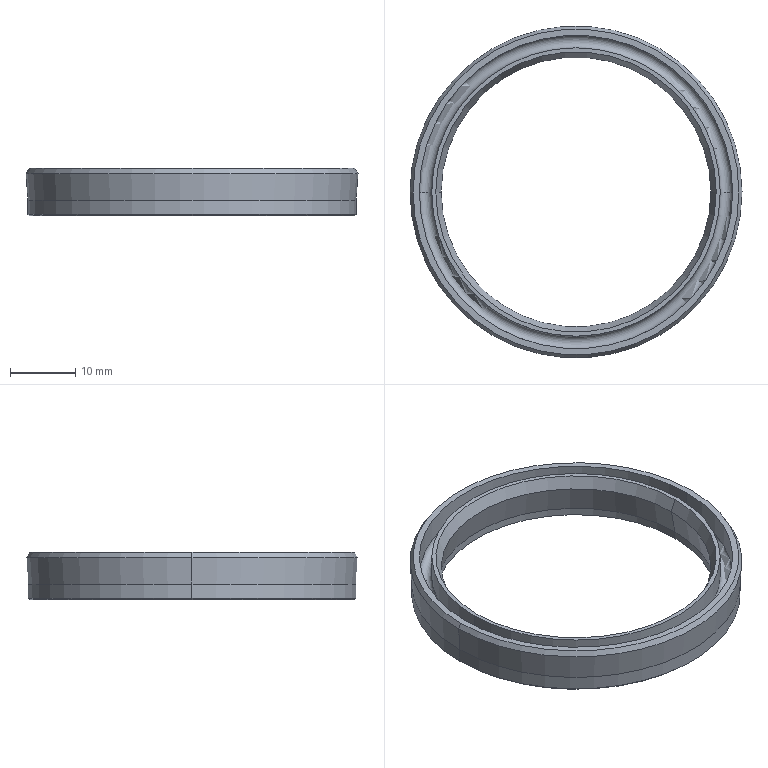Part | NX | features REVOLVE2 2 | 1 solid | 23 faces | box 50.8 x 50.8 x 7.235 mm | volume 3150 mm3 | cone 10 | cylinder 8 | plane 3 | torus 2 | commonest cylinder face diameters 42.799 x2 44.133 x2 47.943 x2 50.228 x2
STEP:
#1=CARTESIAN_POINT('',(25.114,0.,-1.59));
#2=VERTEX_POINT('',#1);
#3=CARTESIAN_POINT('',(-25.114,0.,-1.59));
#4=VERTEX_POINT('',#3);
#5=CARTESIAN_POINT('',(0.,0.,-1.59));
#6=DIRECTION('',(0.,0.,1.));
#7=DIRECTION('',(1.,0.,0.));
#8=AXIS2_PLACEMENT_3D('',#5,#6,#7);
#9=CIRCLE('',#8,25.114);
#10=EDGE_CURVE('',#2,#4,#9,.T.);
#11=ORIENTED_EDGE('',*,*,#10,.T.);
#12=CARTESIAN_POINT('',(-25.4,0.,2.465));
#13=VERTEX_POINT('',#12);
#14=CARTESIAN_POINT('',(-25.114,0.,-1.59));
#15=DIRECTION('',(-0.0703,0.,0.9975));
#16=VECTOR('',#15,1000.);
#17=LINE('',#14,#16);
#18=EDGE_CURVE('',#13,#4,#17,.F.);
#19=ORIENTED_EDGE('',*,*,#18,.F.);
#20=CARTESIAN_POINT('',(25.4,0.,2.465));
#21=VERTEX_POINT('',#20);
#22=CARTESIAN_POINT('',(0.,0.,2.465));
#23=DIRECTION('',(0.,0.,1.));
#24=DIRECTION('',(1.,0.,0.));
#25=AXIS2_PLACEMENT_3D('',#22,#23,#24);
#26=CIRCLE('',#25,25.4);
#27=EDGE_CURVE('',#21,#13,#26,.T.);
#28=ORIENTED_EDGE('',*,*,#27,.F.);
#29=CARTESIAN_POINT('',(25.114,0.,-1.59));
#30=DIRECTION('',(0.0703,0.,0.9975));
#31=VECTOR('',#30,1000.);
#32=LINE('',#29,#31);
#33=EDGE_CURVE('',#2,#21,#32,.T.);
#34=ORIENTED_EDGE('',*,*,#33,.F.);
#35=EDGE_LOOP('',(#11,#19,#28,#34));
#36=FACE_BOUND('',#35,.T.);
#37=CARTESIAN_POINT('',(0.,0.,-1.59));
#38=DIRECTION('',(0.,0.,1.));
#39=DIRECTION('',(-1.,0.,0.));
#40=AXIS2_PLACEMENT_3D('',#37,#38,#39);
#41=CONICAL_SURFACE('',#40,25.114,0.07036);
#42=ADVANCED_FACE('',(#36),#41,.T.);
#43=CARTESIAN_POINT('',(25.114,0.,-3.737));
#44=VERTEX_POINT('',#43);
#45=CARTESIAN_POINT('',(-25.114,0.,-3.737));
#46=VERTEX_POINT('',#45);
#47=CARTESIAN_POINT('',(0.,0.,-3.737));
#48=DIRECTION('',(0.,0.,1.));
#49=DIRECTION('',(1.,0.,0.));
#50=AXIS2_PLACEMENT_3D('',#47,#48,#49);
#51=CIRCLE('',#50,25.114);
#52=EDGE_CURVE('',#44,#46,#51,.T.);
#53=ORIENTED_EDGE('',*,*,#52,.T.);
#54=CARTESIAN_POINT('',(-25.114,0.,3.975));
#55=DIRECTION('',(0.,0.,1.));
#56=VECTOR('',#55,1000.);
#57=LINE('',#54,#56);
#58=EDGE_CURVE('',#46,#4,#57,.T.);
#59=ORIENTED_EDGE('',*,*,#58,.T.);
#60=ORIENTED_EDGE('',*,*,#10,.F.);
#61=CARTESIAN_POINT('',(25.114,0.,3.975));
#62=DIRECTION('',(0.,0.,1.));
#63=VECTOR('',#62,1000.);
#64=LINE('',#61,#63);
#65=EDGE_CURVE('',#2,#44,#64,.F.);
#66=ORIENTED_EDGE('',*,*,#65,.T.);
#67=EDGE_LOOP('',(#53,#59,#60,#66));
#68=FACE_BOUND('',#67,.T.);
#69=CARTESIAN_POINT('',(0.,0.,3.975));
#70=DIRECTION('',(0.,0.,1.));
#71=DIRECTION('',(-1.,0.,0.));
#72=AXIS2_PLACEMENT_3D('',#69,#70,#71);
#73=CYLINDRICAL_SURFACE('',#72,25.114);
#74=ADVANCED_FACE('',(#68),#73,.T.);
#75=CARTESIAN_POINT('',(24.876,0.,-3.975));
#76=VERTEX_POINT('',#75);
#77=CARTESIAN_POINT('',(-24.876,0.,-3.975));
#78=VERTEX_POINT('',#77);
#79=CARTESIAN_POINT('',(0.,0.,-3.975));
#80=DIRECTION('',(0.,0.,1.));
#81=DIRECTION('',(1.,0.,0.));
#82=AXIS2_PLACEMENT_3D('',#79,#80,#81);
#83=CIRCLE('',#82,24.876);
#84=EDGE_CURVE('',#76,#78,#83,.T.);
#85=ORIENTED_EDGE('',*,*,#84,.T.);
#86=CARTESIAN_POINT('',(-24.876,0.,-3.975));
#87=DIRECTION('',(-0.7071,0.,0.7071));
#88=VECTOR('',#87,1000.);
#89=LINE('',#86,#88);
#90=EDGE_CURVE('',#78,#46,#89,.T.);
#91=ORIENTED_EDGE('',*,*,#90,.T.);
#92=ORIENTED_EDGE('',*,*,#52,.F.);
#93=CARTESIAN_POINT('',(24.876,0.,-3.975));
#94=DIRECTION('',(0.7071,0.,0.7071));
#95=VECTOR('',#94,1000.);
#96=LINE('',#93,#95);
#97=EDGE_CURVE('',#44,#76,#96,.F.);
#98=ORIENTED_EDGE('',*,*,#97,.T.);
#99=EDGE_LOOP('',(#85,#91,#92,#98));
#100=FACE_BOUND('',#99,.T.);
#101=CARTESIAN_POINT('',(0.,0.,-3.975));
#102=DIRECTION('',(0.,0.,1.));
#103=DIRECTION('',(-1.,0.,0.));
#104=AXIS2_PLACEMENT_3D('',#101,#102,#103);
#105=CONICAL_SURFACE('',#104,24.876,0.7854);
#106=ADVANCED_FACE('',(#100),#105,.T.);
#107=CARTESIAN_POINT('',(-21.399,0.,-3.975));
#108=VERTEX_POINT('',#107);
#109=CARTESIAN_POINT('',(21.399,0.,-3.975));
#110=VERTEX_POINT('',#109);
#111=CARTESIAN_POINT('',(0.,0.,-3.975));
#112=DIRECTION('',(0.,0.,1.));
#113=DIRECTION('',(1.,0.,0.));
#114=AXIS2_PLACEMENT_3D('',#111,#112,#113);
#115=CIRCLE('',#114,21.399);
#116=EDGE_CURVE('',#108,#110,#115,.T.);
#117=ORIENTED_EDGE('',*,*,#116,.F.);
#118=CARTESIAN_POINT('',(-21.399,0.,-2.783));
#119=VERTEX_POINT('',#118);
#120=CARTESIAN_POINT('',(-21.399,0.,3.975));
#121=DIRECTION('',(0.,0.,1.));
#122=VECTOR('',#121,1000.);
#123=LINE('',#120,#122);
#124=EDGE_CURVE('',#108,#119,#123,.T.);
#125=ORIENTED_EDGE('',*,*,#124,.T.);
#126=CARTESIAN_POINT('',(21.399,0.,-2.783));
#127=VERTEX_POINT('',#126);
#128=CARTESIAN_POINT('',(0.,0.,-2.783));
#129=DIRECTION('',(0.,0.,1.));
#130=DIRECTION('',(1.,0.,0.));
#131=AXIS2_PLACEMENT_3D('',#128,#129,#130);
#132=CIRCLE('',#131,21.399);
#133=EDGE_CURVE('',#119,#127,#132,.T.);
#134=ORIENTED_EDGE('',*,*,#133,.T.);
#135=CARTESIAN_POINT('',(21.399,0.,3.975));
#136=DIRECTION('',(0.,0.,1.));
#137=VECTOR('',#136,1000.);
#138=LINE('',#135,#137);
#139=EDGE_CURVE('',#127,#110,#138,.F.);
#140=ORIENTED_EDGE('',*,*,#139,.T.);
#141=EDGE_LOOP('',(#117,#125,#134,#140));
#142=FACE_BOUND('',#141,.T.);
#143=CARTESIAN_POINT('',(0.,0.,3.975));
#144=DIRECTION('',(0.,0.,1.));
#145=DIRECTION('',(-1.,0.,0.));
#146=AXIS2_PLACEMENT_3D('',#143,#144,#145);
#147=CYLINDRICAL_SURFACE('',#146,21.399);
#148=ADVANCED_FACE('',(#142),#147,.F.);
#149=CARTESIAN_POINT('',(-20.637,0.,1.391));
#150=VERTEX_POINT('',#149);
#151=CARTESIAN_POINT('',(20.637,0.,1.391));
#152=VERTEX_POINT('',#151);
#153=CARTESIAN_POINT('',(0.,0.,1.391));
#154=DIRECTION('',(0.,0.,1.));
#155=DIRECTION('',(1.,0.,0.));
#156=AXIS2_PLACEMENT_3D('',#153,#154,#155);
#157=CIRCLE('',#156,20.637);
#158=EDGE_CURVE('',#150,#152,#157,.T.);
#159=ORIENTED_EDGE('',*,*,#158,.T.);
#160=CARTESIAN_POINT('',(20.637,0.,1.391));
#161=DIRECTION('',(0.1796,0.,-0.9837));
#162=VECTOR('',#161,1000.);
#163=LINE('',#160,#162);
#164=EDGE_CURVE('',#152,#127,#163,.T.);
#165=ORIENTED_EDGE('',*,*,#164,.T.);
#166=ORIENTED_EDGE('',*,*,#133,.F.);
#167=CARTESIAN_POINT('',(-20.637,0.,1.391));
#168=DIRECTION('',(-0.1796,0.,-0.9837));
#169=VECTOR('',#168,1000.);
#170=LINE('',#167,#169);
#171=EDGE_CURVE('',#119,#150,#170,.F.);
#172=ORIENTED_EDGE('',*,*,#171,.T.);
#173=EDGE_LOOP('',(#159,#165,#166,#172));
#174=FACE_BOUND('',#173,.T.);
#175=CARTESIAN_POINT('',(0.,0.,1.391));
#176=DIRECTION('',(0.,0.,-1.));
#177=DIRECTION('',(1.,0.,0.));
#178=AXIS2_PLACEMENT_3D('',#175,#176,#177);
#179=CONICAL_SURFACE('',#178,20.637,0.1806);
#180=ADVANCED_FACE('',(#174),#179,.F.);
#181=ORIENTED_EDGE('',*,*,#158,.F.);
#182=CARTESIAN_POINT('',(-21.447,0.,3.26));
#183=VERTEX_POINT('',#182);
#184=CARTESIAN_POINT('',(-21.447,0.,3.26));
#185=DIRECTION('',(-0.3976,0.,0.9176));
#186=VECTOR('',#185,1000.);
#187=LINE('',#184,#186);
#188=EDGE_CURVE('',#183,#150,#187,.F.);
#189=ORIENTED_EDGE('',*,*,#188,.F.);
#190=CARTESIAN_POINT('',(21.447,0.,3.26));
#191=VERTEX_POINT('',#190);
#192=CARTESIAN_POINT('',(0.,0.,3.26));
#193=DIRECTION('',(0.,0.,1.));
#194=DIRECTION('',(1.,0.,0.));
#195=AXIS2_PLACEMENT_3D('',#192,#193,#194);
#196=CIRCLE('',#195,21.447);
#197=EDGE_CURVE('',#183,#191,#196,.T.);
#198=ORIENTED_EDGE('',*,*,#197,.T.);
#199=CARTESIAN_POINT('',(21.447,0.,3.26));
#200=DIRECTION('',(0.3976,0.,0.9176));
#201=VECTOR('',#200,1000.);
#202=LINE('',#199,#201);
#203=EDGE_CURVE('',#152,#191,#202,.T.);
#204=ORIENTED_EDGE('',*,*,#203,.F.);
#205=EDGE_LOOP('',(#181,#189,#198,#204));
#206=FACE_BOUND('',#205,.T.);
#207=CARTESIAN_POINT('',(0.,0.,3.26));
#208=DIRECTION('',(0.,0.,1.));
#209=DIRECTION('',(-1.,0.,0.));
#210=AXIS2_PLACEMENT_3D('',#207,#208,#209);
#211=CONICAL_SURFACE('',#210,21.447,0.4089);
#212=ADVANCED_FACE('',(#206),#211,.F.);
#213=CARTESIAN_POINT('',(22.066,0.,-0.24));
#214=VERTEX_POINT('',#213);
#215=CARTESIAN_POINT('',(-22.066,0.,-0.24));
#216=VERTEX_POINT('',#215);
#217=CARTESIAN_POINT('',(0.,0.,-0.24));
#218=DIRECTION('',(0.,0.,1.));
#219=DIRECTION('',(1.,0.,0.));
#220=AXIS2_PLACEMENT_3D('',#217,#218,#219);
#221=CIRCLE('',#220,22.066);
#222=EDGE_CURVE('',#214,#216,#221,.T.);
#223=ORIENTED_EDGE('',*,*,#222,.T.);
#224=CARTESIAN_POINT('',(-22.066,0.,3.26));
#225=VERTEX_POINT('',#224);
#226=CARTESIAN_POINT('',(-22.066,0.,3.975));
#227=DIRECTION('',(0.,0.,1.));
#228=VECTOR('',#227,1000.);
#229=LINE('',#226,#228);
#230=EDGE_CURVE('',#216,#225,#229,.T.);
#231=ORIENTED_EDGE('',*,*,#230,.T.);
#232=CARTESIAN_POINT('',(22.066,0.,3.26));
#233=VERTEX_POINT('',#232);
#234=CARTESIAN_POINT('',(0.,0.,3.26));
#235=DIRECTION('',(0.,0.,1.));
#236=DIRECTION('',(1.,0.,0.));
#237=AXIS2_PLACEMENT_3D('',#234,#235,#236);
#238=CIRCLE('',#237,22.066);
#239=EDGE_CURVE('',#233,#225,#238,.T.);
#240=ORIENTED_EDGE('',*,*,#239,.F.);
#241=CARTESIAN_POINT('',(22.066,0.,3.975));
#242=DIRECTION('',(0.,0.,1.));
#243=VECTOR('',#242,1000.);
#244=LINE('',#241,#243);
#245=EDGE_CURVE('',#233,#214,#244,.F.);
#246=ORIENTED_EDGE('',*,*,#245,.T.);
#247=EDGE_LOOP('',(#223,#231,#240,#246));
#248=FACE_BOUND('',#247,.T.);
#249=CARTESIAN_POINT('',(0.,0.,3.975));
#250=DIRECTION('',(0.,0.,1.));
#251=DIRECTION('',(-1.,0.,0.));
#252=AXIS2_PLACEMENT_3D('',#249,#250,#251);
#253=CYLINDRICAL_SURFACE('',#252,22.066);
#254=ADVANCED_FACE('',(#248),#253,.T.);
#255=CARTESIAN_POINT('',(0.,0.,-0.24));
#256=DIRECTION('',(0.,0.,1.));
#257=DIRECTION('',(1.,0.,0.));
#258=AXIS2_PLACEMENT_3D('',#255,#256,#257);
#259=CIRCLE('',#258,22.066);
#260=EDGE_CURVE('',#216,#214,#259,.T.);
#261=ORIENTED_EDGE('',*,*,#260,.F.);
#262=CARTESIAN_POINT('',(-23.971,0.,-0.24));
#263=VERTEX_POINT('',#262);
#264=CARTESIAN_POINT('',(-23.019,0.,-0.24));
#265=DIRECTION('',(0.,1.,0.));
#266=DIRECTION('',(-1.,0.,0.));
#267=AXIS2_PLACEMENT_3D('',#264,#265,#266);
#268=CIRCLE('',#267,0.9525);
#269=EDGE_CURVE('',#263,#216,#268,.F.);
#270=ORIENTED_EDGE('',*,*,#269,.F.);
#271=CARTESIAN_POINT('',(23.971,0.,-0.24));
#272=VERTEX_POINT('',#271);
#273=CARTESIAN_POINT('',(0.,0.,-0.24));
#274=DIRECTION('',(0.,0.,1.));
#275=DIRECTION('',(1.,0.,0.));
#276=AXIS2_PLACEMENT_3D('',#273,#274,#275);
#277=CIRCLE('',#276,23.971);
#278=EDGE_CURVE('',#263,#272,#277,.T.);
#279=ORIENTED_EDGE('',*,*,#278,.T.);
#280=CARTESIAN_POINT('',(23.019,0.,-0.24));
#281=DIRECTION('',(0.,-1.,0.));
#282=DIRECTION('',(0.,0.,-1.));
#283=AXIS2_PLACEMENT_3D('',#280,#281,#282);
#284=CIRCLE('',#283,0.9525);
#285=EDGE_CURVE('',#214,#272,#284,.T.);
#286=ORIENTED_EDGE('',*,*,#285,.F.);
#287=EDGE_LOOP('',(#261,#270,#279,#286));
#288=FACE_BOUND('',#287,.T.);
#289=CARTESIAN_POINT('',(0.,0.,-0.24));
#290=DIRECTION('',(0.,0.,1.));
#291=DIRECTION('',(-1.,0.,0.));
#292=AXIS2_PLACEMENT_3D('',#289,#290,#291);
#293=TOROIDAL_SURFACE('',#292,23.019,0.9525);
#294=ADVANCED_FACE('',(#288),#293,.F.);
#295=ORIENTED_EDGE('',*,*,#278,.F.);
#296=CARTESIAN_POINT('',(-23.971,0.,3.26));
#297=VERTEX_POINT('',#296);
#298=CARTESIAN_POINT('',(-23.971,0.,3.975));
#299=DIRECTION('',(0.,0.,1.));
#300=VECTOR('',#299,1000.);
#301=LINE('',#298,#300);
#302=EDGE_CURVE('',#263,#297,#301,.T.);
#303=ORIENTED_EDGE('',*,*,#302,.T.);
#304=CARTESIAN_POINT('',(23.971,0.,3.26));
#305=VERTEX_POINT('',#304);
#306=CARTESIAN_POINT('',(0.,0.,3.26));
#307=DIRECTION('',(0.,0.,1.));
#308=DIRECTION('',(1.,0.,0.));
#309=AXIS2_PLACEMENT_3D('',#306,#307,#308);
#310=CIRCLE('',#309,23.971);
#311=EDGE_CURVE('',#297,#305,#310,.T.);
#312=ORIENTED_EDGE('',*,*,#311,.T.);
#313=CARTESIAN_POINT('',(23.971,0.,3.975));
#314=DIRECTION('',(0.,0.,1.));
#315=VECTOR('',#314,1000.);
#316=LINE('',#313,#315);
#317=EDGE_CURVE('',#305,#272,#316,.F.);
#318=ORIENTED_EDGE('',*,*,#317,.T.);
#319=EDGE_LOOP('',(#295,#303,#312,#318));
#320=FACE_BOUND('',#319,.T.);
#321=CARTESIAN_POINT('',(0.,0.,3.975));
#322=DIRECTION('',(0.,0.,1.));
#323=DIRECTION('',(-1.,0.,0.));
#324=AXIS2_PLACEMENT_3D('',#321,#322,#323);
#325=CYLINDRICAL_SURFACE('',#324,23.971);
#326=ADVANCED_FACE('',(#320),#325,.F.);
#327=CARTESIAN_POINT('',(24.924,0.,3.26));
#328=VERTEX_POINT('',#327);
#329=CARTESIAN_POINT('',(-24.924,0.,3.26));
#330=VERTEX_POINT('',#329);
#331=CARTESIAN_POINT('',(0.,0.,3.26));
#332=DIRECTION('',(0.,0.,1.));
#333=DIRECTION('',(1.,0.,0.));
#334=AXIS2_PLACEMENT_3D('',#331,#332,#333);
#335=CIRCLE('',#334,24.924);
#336=EDGE_CURVE('',#328,#330,#335,.T.);
#337=ORIENTED_EDGE('',*,*,#336,.F.);
#338=CARTESIAN_POINT('',(25.4,0.,2.465));
#339=DIRECTION('',(0.5139,0.,-0.8579));
#340=VECTOR('',#339,1000.);
#341=LINE('',#338,#340);
#342=EDGE_CURVE('',#21,#328,#341,.F.);
#343=ORIENTED_EDGE('',*,*,#342,.F.);
#344=ORIENTED_EDGE('',*,*,#27,.T.);
#345=CARTESIAN_POINT('',(-25.4,0.,2.465));
#346=DIRECTION('',(-0.5139,0.,-0.8579));
#347=VECTOR('',#346,1000.);
#348=LINE('',#345,#347);
#349=EDGE_CURVE('',#330,#13,#348,.T.);
#350=ORIENTED_EDGE('',*,*,#349,.F.);
#351=EDGE_LOOP('',(#337,#343,#344,#350));
#352=FACE_BOUND('',#351,.T.);
#353=CARTESIAN_POINT('',(0.,0.,2.465));
#354=DIRECTION('',(0.,0.,-1.));
#355=DIRECTION('',(1.,0.,0.));
#356=AXIS2_PLACEMENT_3D('',#353,#354,#355);
#357=CONICAL_SURFACE('',#356,25.4,0.5397);
#358=ADVANCED_FACE('',(#352),#357,.T.);
#359=ORIENTED_EDGE('',*,*,#342,.T.);
#360=CARTESIAN_POINT('',(0.,0.,3.26));
#361=DIRECTION('',(0.,0.,1.));
#362=DIRECTION('',(1.,0.,0.));
#363=AXIS2_PLACEMENT_3D('',#360,#361,#362);
#364=CIRCLE('',#363,24.924);
#365=EDGE_CURVE('',#330,#328,#364,.T.);
#366=ORIENTED_EDGE('',*,*,#365,.F.);
#367=ORIENTED_EDGE('',*,*,#349,.T.);
#368=CARTESIAN_POINT('',(0.,0.,2.465));
#369=DIRECTION('',(0.,0.,1.));
#370=DIRECTION('',(1.,0.,0.));
#371=AXIS2_PLACEMENT_3D('',#368,#369,#370);
#372=CIRCLE('',#371,25.4);
#373=EDGE_CURVE('',#13,#21,#372,.T.);
#374=ORIENTED_EDGE('',*,*,#373,.T.);
#375=EDGE_LOOP('',(#359,#366,#367,#374));
#376=FACE_BOUND('',#375,.T.);
#377=CARTESIAN_POINT('',(0.,0.,2.465));
#378=DIRECTION('',(0.,0.,-1.));
#379=DIRECTION('',(1.,0.,0.));
#380=AXIS2_PLACEMENT_3D('',#377,#378,#379);
#381=CONICAL_SURFACE('',#380,25.4,0.5397);
#382=ADVANCED_FACE('',(#376),#381,.T.);
#383=CARTESIAN_POINT('',(0.,0.,3.26));
#384=DIRECTION('',(0.,0.,1.));
#385=DIRECTION('',(1.,0.,0.));
#386=AXIS2_PLACEMENT_3D('',#383,#384,#385);
#387=CIRCLE('',#386,23.971);
#388=EDGE_CURVE('',#305,#297,#387,.T.);
#389=ORIENTED_EDGE('',*,*,#388,.F.);
#390=ORIENTED_EDGE('',*,*,#311,.F.);
#391=EDGE_LOOP('',(#389,#390));
#392=FACE_BOUND('',#391,.T.);
#393=ORIENTED_EDGE('',*,*,#365,.T.);
#394=ORIENTED_EDGE('',*,*,#336,.T.);
#395=EDGE_LOOP('',(#393,#394));
#396=FACE_BOUND('',#395,.T.);
#397=CARTESIAN_POINT('',(0.,24.924,3.26));
#398=DIRECTION('',(0.,0.,-1.));
#399=DIRECTION('',(1.,0.,0.));
#400=AXIS2_PLACEMENT_3D('',#397,#398,#399);
#401=PLANE('',#400);
#402=ADVANCED_FACE('',(#392,#396),#401,.F.);
#403=ORIENTED_EDGE('',*,*,#302,.F.);
#404=CARTESIAN_POINT('',(0.,0.,-0.24));
#405=DIRECTION('',(0.,0.,1.));
#406=DIRECTION('',(1.,0.,0.));
#407=AXIS2_PLACEMENT_3D('',#404,#405,#406);
#408=CIRCLE('',#407,23.971);
#409=EDGE_CURVE('',#272,#263,#408,.T.);
#410=ORIENTED_EDGE('',*,*,#409,.F.);
#411=ORIENTED_EDGE('',*,*,#317,.F.);
#412=ORIENTED_EDGE('',*,*,#388,.T.);
#413=EDGE_LOOP('',(#403,#410,#411,#412));
#414=FACE_BOUND('',#413,.T.);
#415=CARTESIAN_POINT('',(0.,0.,3.975));
#416=DIRECTION('',(0.,0.,1.));
#417=DIRECTION('',(-1.,0.,0.));
#418=AXIS2_PLACEMENT_3D('',#415,#416,#417);
#419=CYLINDRICAL_SURFACE('',#418,23.971);
#420=ADVANCED_FACE('',(#414),#419,.F.);
#421=ORIENTED_EDGE('',*,*,#269,.T.);
#422=ORIENTED_EDGE('',*,*,#222,.F.);
#423=ORIENTED_EDGE('',*,*,#285,.T.);
#424=ORIENTED_EDGE('',*,*,#409,.T.);
#425=EDGE_LOOP('',(#421,#422,#423,#424));
#426=FACE_BOUND('',#425,.T.);
#427=CARTESIAN_POINT('',(0.,0.,-0.24));
#428=DIRECTION('',(0.,0.,1.));
#429=DIRECTION('',(-1.,0.,0.));
#430=AXIS2_PLACEMENT_3D('',#427,#428,#429);
#431=TOROIDAL_SURFACE('',#430,23.019,0.9525);
#432=ADVANCED_FACE('',(#426),#431,.F.);
#433=ORIENTED_EDGE('',*,*,#230,.F.);
#434=ORIENTED_EDGE('',*,*,#260,.T.);
#435=ORIENTED_EDGE('',*,*,#245,.F.);
#436=CARTESIAN_POINT('',(0.,0.,3.26));
#437=DIRECTION('',(0.,0.,1.));
#438=DIRECTION('',(1.,0.,0.));
#439=AXIS2_PLACEMENT_3D('',#436,#437,#438);
#440=CIRCLE('',#439,22.066);
#441=EDGE_CURVE('',#225,#233,#440,.T.);
#442=ORIENTED_EDGE('',*,*,#441,.F.);
#443=EDGE_LOOP('',(#433,#434,#435,#442));
#444=FACE_BOUND('',#443,.T.);
#445=CARTESIAN_POINT('',(0.,0.,3.975));
#446=DIRECTION('',(0.,0.,1.));
#447=DIRECTION('',(-1.,0.,0.));
#448=AXIS2_PLACEMENT_3D('',#445,#446,#447);
#449=CYLINDRICAL_SURFACE('',#448,22.066);
#450=ADVANCED_FACE('',(#444),#449,.T.);
#451=CARTESIAN_POINT('',(0.,0.,3.26));
#452=DIRECTION('',(0.,0.,1.));
#453=DIRECTION('',(1.,0.,0.));
#454=AXIS2_PLACEMENT_3D('',#451,#452,#453);
#455=CIRCLE('',#454,21.447);
#456=EDGE_CURVE('',#191,#183,#455,.T.);
#457=ORIENTED_EDGE('',*,*,#456,.F.);
#458=ORIENTED_EDGE('',*,*,#197,.F.);
#459=EDGE_LOOP('',(#457,#458));
#460=FACE_BOUND('',#459,.T.);
#461=ORIENTED_EDGE('',*,*,#239,.T.);
#462=ORIENTED_EDGE('',*,*,#441,.T.);
#463=EDGE_LOOP('',(#461,#462));
#464=FACE_BOUND('',#463,.T.);
#465=CARTESIAN_POINT('',(0.,21.447,3.26));
#466=DIRECTION('',(0.,0.,-1.));
#467=DIRECTION('',(1.,0.,0.));
#468=AXIS2_PLACEMENT_3D('',#465,#466,#467);
#469=PLANE('',#468);
#470=ADVANCED_FACE('',(#460,#464),#469,.F.);
#471=ORIENTED_EDGE('',*,*,#188,.T.);
#472=CARTESIAN_POINT('',(0.,0.,1.391));
#473=DIRECTION('',(0.,0.,1.));
#474=DIRECTION('',(1.,0.,0.));
#475=AXIS2_PLACEMENT_3D('',#472,#473,#474);
#476=CIRCLE('',#475,20.637);
#477=EDGE_CURVE('',#152,#150,#476,.T.);
#478=ORIENTED_EDGE('',*,*,#477,.F.);
#479=ORIENTED_EDGE('',*,*,#203,.T.);
#480=ORIENTED_EDGE('',*,*,#456,.T.);
#481=EDGE_LOOP('',(#471,#478,#479,#480));
#482=FACE_BOUND('',#481,.T.);
#483=CARTESIAN_POINT('',(0.,0.,3.26));
#484=DIRECTION('',(0.,0.,1.));
#485=DIRECTION('',(-1.,0.,0.));
#486=AXIS2_PLACEMENT_3D('',#483,#484,#485);
#487=CONICAL_SURFACE('',#486,21.447,0.4089);
#488=ADVANCED_FACE('',(#482),#487,.F.);
#489=ORIENTED_EDGE('',*,*,#164,.F.);
#490=ORIENTED_EDGE('',*,*,#477,.T.);
#491=ORIENTED_EDGE('',*,*,#171,.F.);
#492=CARTESIAN_POINT('',(0.,0.,-2.783));
#493=DIRECTION('',(0.,0.,1.));
#494=DIRECTION('',(1.,0.,0.));
#495=AXIS2_PLACEMENT_3D('',#492,#493,#494);
#496=CIRCLE('',#495,21.399);
#497=EDGE_CURVE('',#127,#119,#496,.T.);
#498=ORIENTED_EDGE('',*,*,#497,.F.);
#499=EDGE_LOOP('',(#489,#490,#491,#498));
#500=FACE_BOUND('',#499,.T.);
#501=CARTESIAN_POINT('',(0.,0.,1.391));
#502=DIRECTION('',(0.,0.,-1.));
#503=DIRECTION('',(1.,0.,0.));
#504=AXIS2_PLACEMENT_3D('',#501,#502,#503);
#505=CONICAL_SURFACE('',#504,20.637,0.1806);
#506=ADVANCED_FACE('',(#500),#505,.F.);
#507=ORIENTED_EDGE('',*,*,#124,.F.);
#508=CARTESIAN_POINT('',(0.,0.,-3.975));
#509=DIRECTION('',(0.,0.,1.));
#510=DIRECTION('',(1.,0.,0.));
#511=AXIS2_PLACEMENT_3D('',#508,#509,#510);
#512=CIRCLE('',#511,21.399);
#513=EDGE_CURVE('',#110,#108,#512,.T.);
#514=ORIENTED_EDGE('',*,*,#513,.F.);
#515=ORIENTED_EDGE('',*,*,#139,.F.);
#516=ORIENTED_EDGE('',*,*,#497,.T.);
#517=EDGE_LOOP('',(#507,#514,#515,#516));
#518=FACE_BOUND('',#517,.T.);
#519=CARTESIAN_POINT('',(0.,0.,3.975));
#520=DIRECTION('',(0.,0.,1.));
#521=DIRECTION('',(-1.,0.,0.));
#522=AXIS2_PLACEMENT_3D('',#519,#520,#521);
#523=CYLINDRICAL_SURFACE('',#522,21.399);
#524=ADVANCED_FACE('',(#518),#523,.F.);
#525=ORIENTED_EDGE('',*,*,#84,.F.);
#526=CARTESIAN_POINT('',(0.,0.,-3.975));
#527=DIRECTION('',(0.,0.,1.));
#528=DIRECTION('',(1.,0.,0.));
#529=AXIS2_PLACEMENT_3D('',#526,#527,#528);
#530=CIRCLE('',#529,24.876);
#531=EDGE_CURVE('',#78,#76,#530,.T.);
#532=ORIENTED_EDGE('',*,*,#531,.F.);
#533=EDGE_LOOP('',(#525,#532));
#534=FACE_BOUND('',#533,.T.);
#535=ORIENTED_EDGE('',*,*,#513,.T.);
#536=ORIENTED_EDGE('',*,*,#116,.T.);
#537=EDGE_LOOP('',(#535,#536));
#538=FACE_BOUND('',#537,.T.);
#539=CARTESIAN_POINT('',(0.,24.876,-3.975));
#540=DIRECTION('',(0.,0.,1.));
#541=DIRECTION('',(-1.,0.,0.));
#542=AXIS2_PLACEMENT_3D('',#539,#540,#541);
#543=PLANE('',#542);
#544=ADVANCED_FACE('',(#534,#538),#543,.F.);
#545=ORIENTED_EDGE('',*,*,#90,.F.);
#546=ORIENTED_EDGE('',*,*,#531,.T.);
#547=ORIENTED_EDGE('',*,*,#97,.F.);
#548=CARTESIAN_POINT('',(0.,0.,-3.737));
#549=DIRECTION('',(0.,0.,1.));
#550=DIRECTION('',(1.,0.,0.));
#551=AXIS2_PLACEMENT_3D('',#548,#549,#550);
#552=CIRCLE('',#551,25.114);
#553=EDGE_CURVE('',#46,#44,#552,.T.);
#554=ORIENTED_EDGE('',*,*,#553,.F.);
#555=EDGE_LOOP('',(#545,#546,#547,#554));
#556=FACE_BOUND('',#555,.T.);
#557=CARTESIAN_POINT('',(0.,0.,-3.975));
#558=DIRECTION('',(0.,0.,1.));
#559=DIRECTION('',(-1.,0.,0.));
#560=AXIS2_PLACEMENT_3D('',#557,#558,#559);
#561=CONICAL_SURFACE('',#560,24.876,0.7854);
#562=ADVANCED_FACE('',(#556),#561,.T.);
#563=ORIENTED_EDGE('',*,*,#58,.F.);
#564=ORIENTED_EDGE('',*,*,#553,.T.);
#565=ORIENTED_EDGE('',*,*,#65,.F.);
#566=CARTESIAN_POINT('',(0.,0.,-1.59));
#567=DIRECTION('',(0.,0.,1.));
#568=DIRECTION('',(1.,0.,0.));
#569=AXIS2_PLACEMENT_3D('',#566,#567,#568);
#570=CIRCLE('',#569,25.114);
#571=EDGE_CURVE('',#4,#2,#570,.T.);
#572=ORIENTED_EDGE('',*,*,#571,.F.);
#573=EDGE_LOOP('',(#563,#564,#565,#572));
#574=FACE_BOUND('',#573,.T.);
#575=CARTESIAN_POINT('',(0.,0.,3.975));
#576=DIRECTION('',(0.,0.,1.));
#577=DIRECTION('',(-1.,0.,0.));
#578=AXIS2_PLACEMENT_3D('',#575,#576,#577);
#579=CYLINDRICAL_SURFACE('',#578,25.114);
#580=ADVANCED_FACE('',(#574),#579,.T.);
#581=ORIENTED_EDGE('',*,*,#18,.T.);
#582=ORIENTED_EDGE('',*,*,#571,.T.);
#583=ORIENTED_EDGE('',*,*,#33,.T.);
#584=ORIENTED_EDGE('',*,*,#373,.F.);
#585=EDGE_LOOP('',(#581,#582,#583,#584));
#586=FACE_BOUND('',#585,.T.);
#587=CARTESIAN_POINT('',(0.,0.,-1.59));
#588=DIRECTION('',(0.,0.,1.));
#589=DIRECTION('',(-1.,0.,0.));
#590=AXIS2_PLACEMENT_3D('',#587,#588,#589);
#591=CONICAL_SURFACE('',#590,25.114,0.07036);
#592=ADVANCED_FACE('',(#586),#591,.T.);
#593=CLOSED_SHELL('',(#42,#74,#106,#148,#180,#212,#254,#294,#326,#358,#382,#402,#420,#432,#450,#470,#488,#506,#524,#544,#562,#580,#592));
#594=MANIFOLD_SOLID_BREP('',#593);
#595=(LENGTH_UNIT()NAMED_UNIT(*)SI_UNIT(.MILLI.,.METRE.));
#596=UNCERTAINTY_MEASURE_WITH_UNIT(LENGTH_MEASURE(0.00001),#595,'','');
#597=(NAMED_UNIT(*)PLANE_ANGLE_UNIT()SI_UNIT($,.RADIAN.));
#598=(NAMED_UNIT(*)SI_UNIT($,.STERADIAN.)SOLID_ANGLE_UNIT());
#599=(GEOMETRIC_REPRESENTATION_CONTEXT(3)GLOBAL_UNCERTAINTY_ASSIGNED_CONTEXT((#596))GLOBAL_UNIT_ASSIGNED_CONTEXT((#595,#597,#598))REPRESENTATION_CONTEXT('',''));
#600=ADVANCED_BREP_SHAPE_REPRESENTATION('',(#594),#599);